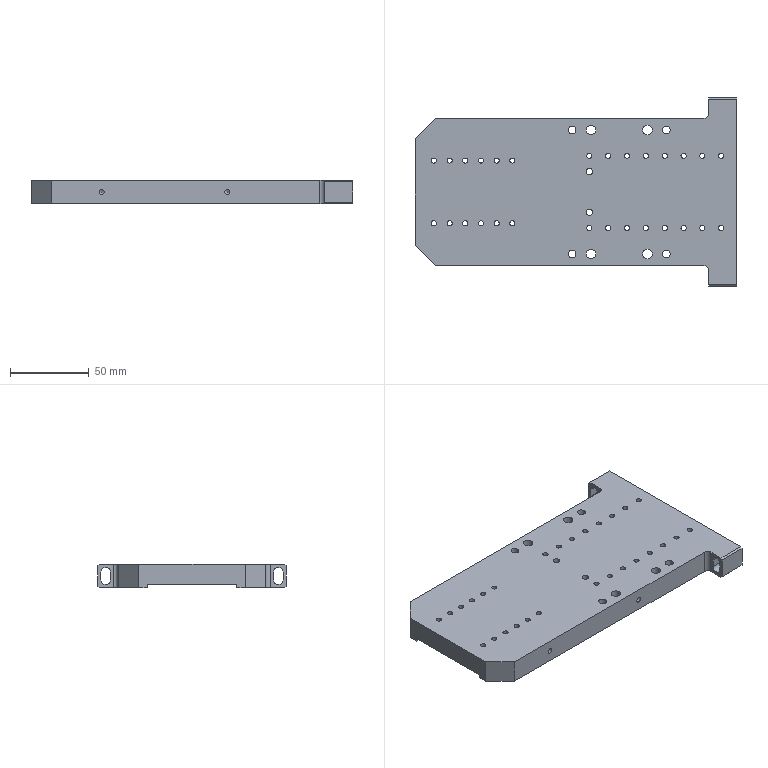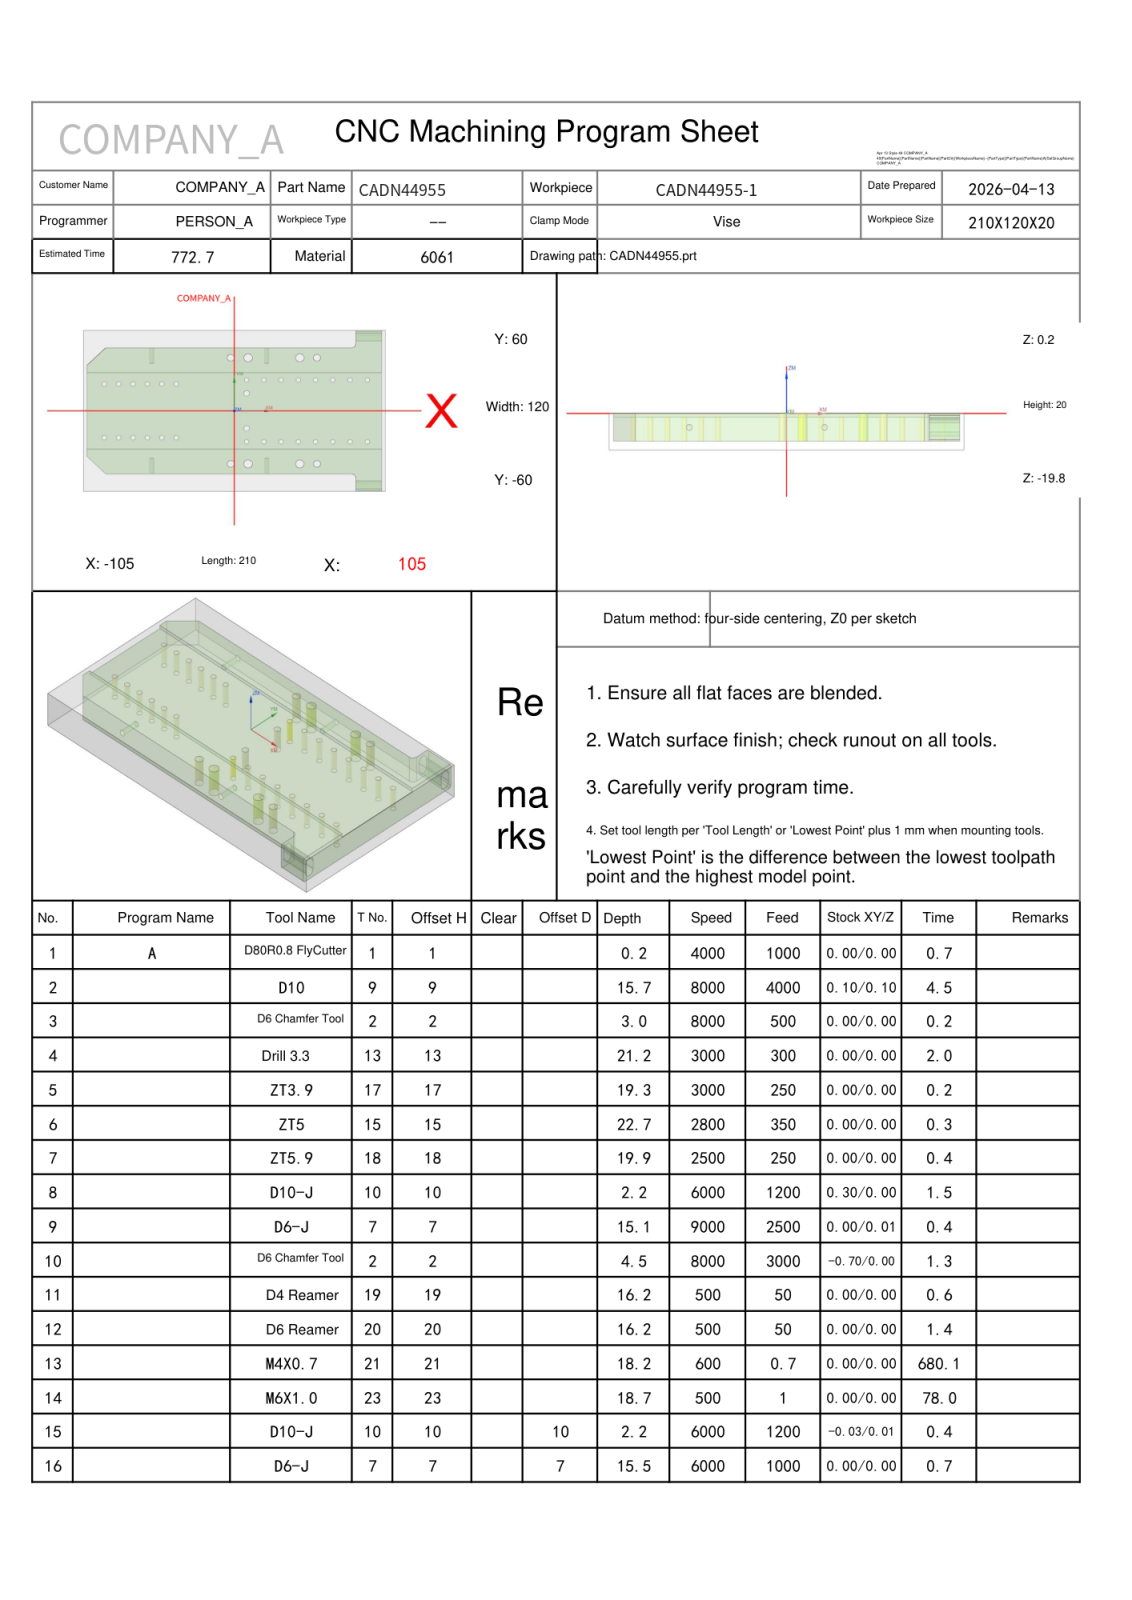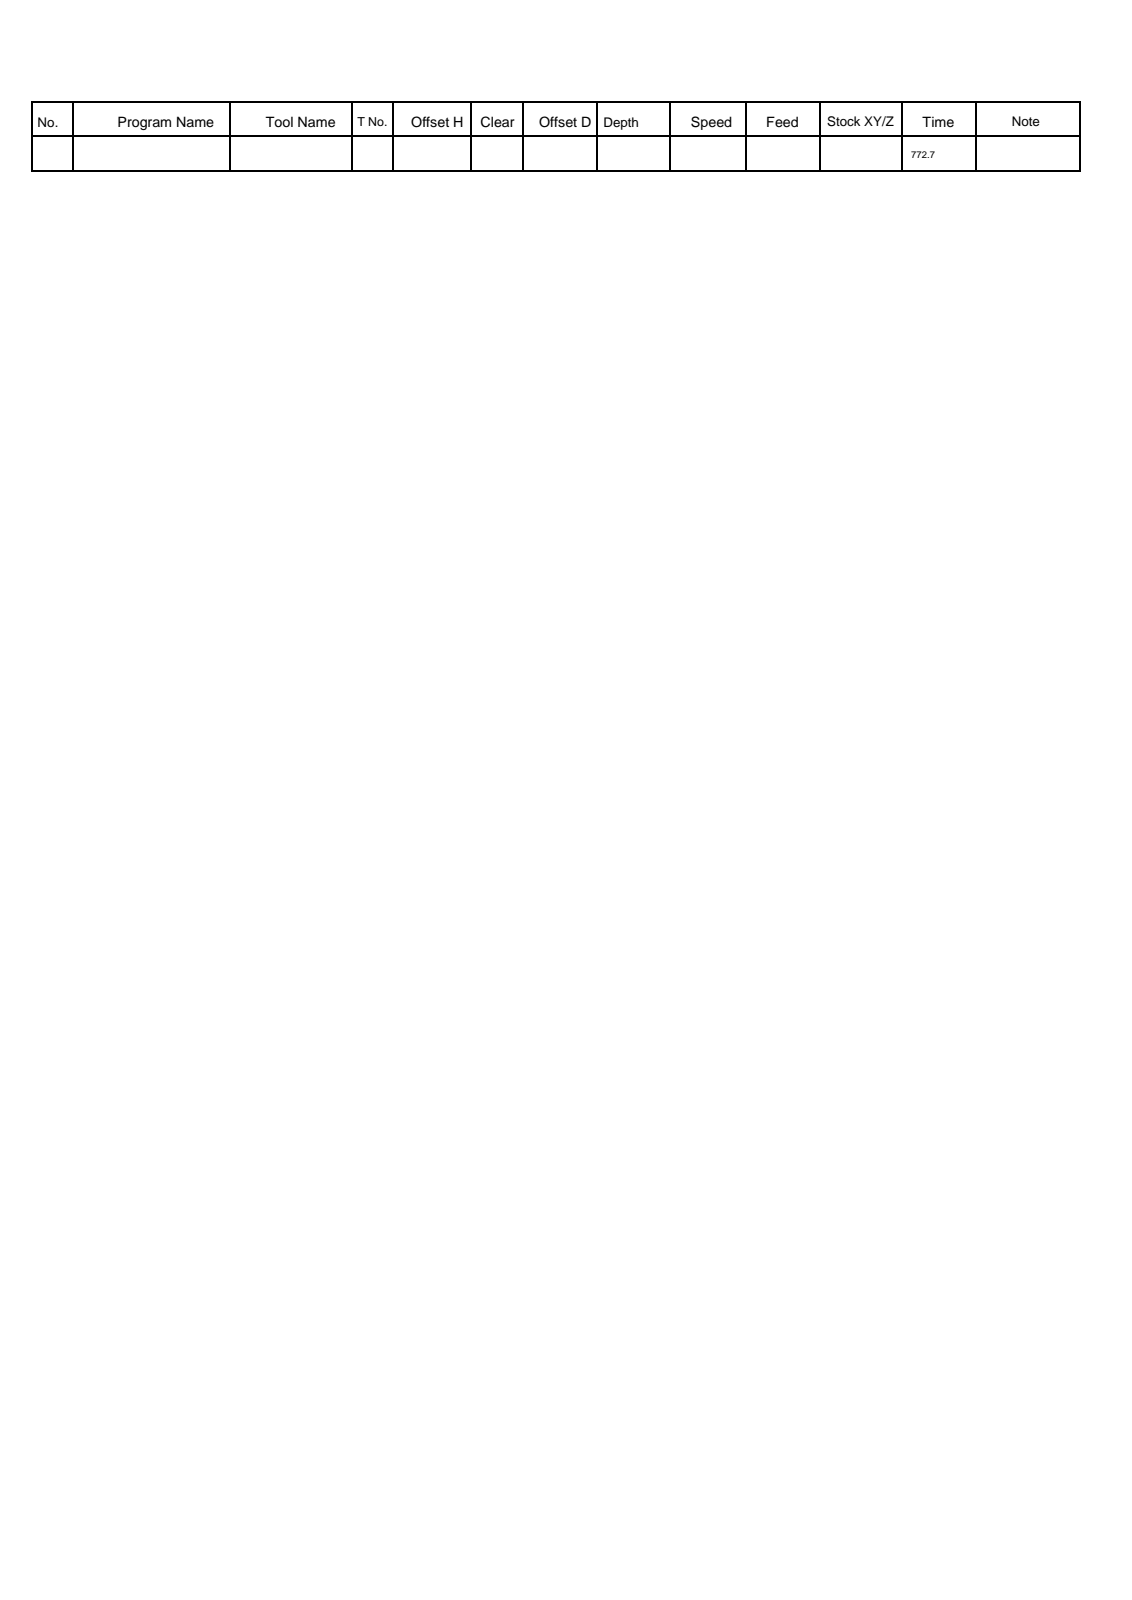NC program | NX | posted by the shop | part box 205 x 120 x 15 mm
Lines 1 to 1265 of 4760:
%
O0001
(Machine time: 1489.33 MIN)
(===Total Tool:13===)
(T1=D80R0.8 FlyCutter D=80.  R=0.8  D-  H01 Z=-0.   )
(T9=D10     D=10.  R=0.   D-  H09 Z=-15.5 )
(T2=D6 ChamferTool   D=6.   R=0.   D-  H02 Z=-4.3  )
(T13=Drill 3.3  D=3.3  DR_a=118 D-  H13 Z=-20.99)
(T17=ZT3.9  D=3.9  DR_a=120 D-  H17 Z=-19.13)
(T15=ZT5    D=5.   DR_a=118 D-  H15 Z=-22.5 )
(T18=ZT5.9  D=5.9  DR_a=120 D-  H18 Z=-19.7 )
(T10=D10-J  D=10.  R=0.   D-  H10 Z=-2.   )
(T7=D6-J    D=6.   R=0.   D-  H07 Z=-15.3 )
(T19=D4 Reamer   D=4.   DR_a=180 D-  H19 Z=-16.  )
(T20=D6 Reamer   D=6.   DR_a=180 D-  H20 Z=-16.  )
(T21=M4X0.7 D=3.3  DR_a=180 D-  H21 Z=-18.  )
(T23=M6X1.0 D=5.   DR_a=180 D-  H23 Z=-18.5 )
G80 G90 G17 G49 G40
G91 G28 Z0
M01
N1 T01 M06
(D80R0.8 FlyCutter  D=80. R=0.8 H=01 ce=0.00 di=0.00)
(MAX_Z=20. MIN_Z=-0. Time=0.66M)
G00 G90 G54 X147.5 Y-33.333 M03 S4000
G43 H01 Z20.
M08
Z2.
G01 Z0.0 F1000.
X142.5
X-142.5
Y33.333
X142.5
X147.5
Z2.
G00 Z20.
G91 G28 Z0.0
M05
M09
G91 G28 Z0.0
M01
N2 T09 M06
(D10  D=10. R=0. H=09 ce=0.12 di=0.10)
(MAX_Z=20. MIN_Z=-15.5 Time=4.44M)
G00 G90 G54 X115.931 Y.933 M03 S8000
G43 H09 Z20.
M08
Z-13.5
G01 X115.832 Y.914 Z-14.125 F4000.
X115.734 Y.895 Z-14.372
X115.636 Y.877 Z-14.554
X115.538 Y.858 Z-14.7
X115.439 Y.839 Z-14.823
X115.341 Y.821 Z-14.928
X115.243 Y.802 Z-15.02
X115.145 Y.783 Z-15.1
X115.046 Y.765 Z-15.17
X114.948 Y.746 Z-15.232
X114.85 Y.727 Z-15.286
X114.752 Y.709 Z-15.333
X114.653 Y.69 Z-15.374
X114.555 Y.671 Z-15.408
X114.457 Y.653 Z-15.436
X114.359 Y.634 Z-15.46
X114.261 Y.615 Z-15.477
X114.162 Y.597 Z-15.49
X114.064 Y.578 Z-15.497
X113.966 Y.559 Z-15.5
X111.852 Y.158
G03 X111.5 Y-.101 I.101 J-.505
X110.862 Y-3.914 I12.263 J-4.012
X110.681 Y-14.084 I285.594 J-10.169
X110.7 Y-17.408 I285.775 J0.0
G01 X110.683 Y-58.128
G02 X106.817 Y-64.032 I-6.644 J.133
X101.024 Y-65.449 I-6.598 J14.422
X91.905 Y-65.715 I-9.119 J156.488
X89.509 Y-65.696 I0.0 J156.754
G01 X-103.13 Y-65.682
G02 X-109.102 Y-61.67 I.144 J6.665
X-110.476 Y-55.702 I15.279 J6.659
X-110.719 Y-46.222 I184.586 J9.48
X-110.699 Y-43.467 I184.829 J0.0
G01 X-110.68 Y58.17
G02 X-106.87 Y63.995 I6.601 J-.16
X-101.239 Y65.427 I6.537 J-13.917
X-92.501 Y65.714 I8.738 J-132.999
X-90.366 Y65.697 I0.0 J-133.286
G01 X103.25 Y65.676
G02 X108.958 Y61.949 I-.203 J-6.546
X110.434 Y56.172 I-13.856 J-6.618
X110.713 Y47.477 I-135.526 J-8.695
X110.697 Y45.378 I-135.804 J0.0
G01 X110.683 Y2.679
G03 X110.095 Y-4.195 I455.395 J-42.432
X109.895 Y-14.598 I270.442 J-10.404
X109.9 Y-16.368 I270.642 J0.0
G01 X109.884 Y-56.108
G02 X107.365 Y-61.553 I-7.562 J.194
G01 X106.934 Y-62.56
X106.12 Y-63.62
X105.06 Y-64.434
X103.825 Y-64.946
X102.498 Y-65.12
X84.221 Y-65.098
G03 X75.842 Y-64.892 I-8.378 J-170.229
X73.989 Y-64.902 I0.0 J-170.435
G01 X-101.208 Y-64.879
G02 X-107.674 Y-60.783 I.383 J7.756
X-109.531 Y-54.375 I14.417 J7.651
X-109.905 Y-45.467 I105.986 J8.909
X-109.892 Y-43.826 I106.359 J0.0
G01 X-109.877 Y56.247
G02 X-105.805 Y62.659 I7.751 J-.424
X-99.391 Y64.529 I7.66 J-14.337
X-90.425 Y64.906 I8.966 J-106.458
X-88.762 Y64.893 I0.0 J-106.835
G01 X83.043 Y64.908
X84.502 Y65.12
X102.502
X103.825 Y64.946
X105.06 Y64.434
G02 X107.707 Y61.406 I-4.202 J-6.345
X109.559 Y54.573 I-16.215 J-8.062
X109.899 Y45.806 I-112.829 J-8.767
X109.892 Y44.502 I-113.169 J0.0
G01 X109.873 Y4.122
G02 X109.322 Y-4.177 I-786.201 J48.07
G03 X109.086 Y-17.016 I349.156 J-12.839
X109.101 Y-20.208 I349.392 J0.0
G01 X109.079 Y-54.268
G02 X107.67 Y-59.053 I-11.286 J.725
G03 X107.603 Y-59.683 I2.925 J-.63
X107.62 Y-60.002 I2.992 J0.0
G01 X107.446 Y-61.325
X107.323 Y-61.621
X107.446 Y-61.325
G03 X107.649 Y-58.872 I-17.171 J2.657
X108.438 Y-50.971 I-39.167 J7.902
X108.432 Y-50.313 I-39.956 J0.0
G01 X108.492 Y-11.541
G02 X109.141 Y2.682 I232.868 J-3.495
G03 X109.263 Y11.371 I-309.22 J8.689
X109.258 Y13.081 I-309.342 J0.0
G01 X109.227 Y47.141
G03 X109.231 Y47.792 I-56.575 J.652
X108.633 Y55.991 I-56.578 J0.0
X107.62 Y59.573 I-19.448 J-3.568
X107.446 Y61.325 I-10.322 J-.143
G01 X106.934 Y62.56
X106.12 Y63.62
X106.934 Y62.56
X107.446 Y61.325
G02 X107.641 Y58.913 I-14.765 J-2.412
X107.638 Y58.591 I-14.961 J0.0
X108.451 Y44.13 I-128.221 J-14.461
X108.445 Y42.88 I-129.034 J0.0
G01 X108.436 Y7.38
G02 X107.915 Y-4.166 I-251.422 J5.565
G03 X107.639 Y-20.142 I462.713 J-15.975
X107.661 Y-24.609 I462.988 J0.0
G01 X107.63 Y-49.609
X107.62 Y-59.205
X107.635 Y1.039
G03 X107.83 Y15.095 I-507.419 J14.056
X107.818 Y18.54 I-507.613 J0.0
G01 X107.782 Y45.08
G03 X107.62 Y50.886 I-539.839 J-12.143
G01 Y58.966
Y.326
G03 X107.795 Y-.055 I.513 J.006
G01 X108.582 Y-.726
X110.082 Y-2.005 Z-15.4
X110.581 Y-2.431
X110.642 Y-2.493
X110.691 Y-2.564
X110.727 Y-2.642
X110.749 Y-2.725
X110.757 Y-2.811
Y-63.265
X110.75 Y-63.442
X110.727 Y-63.618
X110.691 Y-63.792
X110.64 Y-63.962
X110.575 Y-64.127
X110.497 Y-64.286
X110.406 Y-64.438
X110.302 Y-64.582
X110.187 Y-64.717
X110.061 Y-64.842
X109.926 Y-64.957
X109.781 Y-65.059
X104.919 Y-68.204
X104.685 Y-68.348
X104.444 Y-68.48
X104.197 Y-68.6
X103.944 Y-68.707
X103.687 Y-68.803
X103.425 Y-68.885
X103.159 Y-68.955
X102.89 Y-69.012
X102.619 Y-69.056
X102.346 Y-69.086
X102.072 Y-69.103
X101.797 Y-69.106
X101.522 Y-69.096
X87.635 Y-68.257
X87.558 Y-68.246
X87.483 Y-68.223
X87.412 Y-68.189
X87.348 Y-68.144
X87.291 Y-68.089
X86.857 Y-67.598
X85.549 Y-66.122 Z-15.5
X84.756 Y-65.234
X84.498 Y-65.12
G02 X82.23 Y-64.654 I.712 J9.228
G03 X76.11 Y-64.146 I-6.12 J-36.62
X75.677 Y-64.149 I0.0 J-37.127
G01 X65.192 Y-64.1
X-99.188 Y-64.083
G02 X-106.881 Y-59.122 I.265 J8.856
X-108.708 Y-52.442 I16.621 J8.136
X-109.102 Y-43.026 I112.211 J9.416
X-109.091 Y-41.414 I112.606 J0.0
G01 X-109.075 Y54.326
G02 X-104.209 Y61.832 I8.829 J-.393
X-97.624 Y63.687 I8.117 J-16.205
X-88.243 Y64.102 I9.381 J-105.829
X-86.677 Y64.09 I0.0 J-106.244
G01 X81.386 Y64.121
G03 X81.94 Y64.434 I-.337 J1.244
G01 X83.175 Y64.946
X81.94 Y64.434
G02 X80.371 Y63.821 I-1.726 J2.105
X74.324 Y63.468 I-6.047 J51.518
X73.378 Y63.476 I0.0 J51.872
G01 X-88.409 Y63.436
G03 X-89.329 Y63.442 I-.92 J-71.028
X-98.066 Y62.902 I0.0 J-71.034
X-104.129 Y60.744 I1.689 J-14.335
X-107.836 Y54.861 I5.345 J-7.477
X-108.422 Y48.3 I36.385 J-6.561
X-108.42 Y47.857 I36.972 J0.0
G01 X-108.458 Y38.897
X-108.436 Y-43.403
G03 X-108.441 Y-44.251 I73.299 J-.847
X-107.928 Y-52.903 I73.304 J0.0
X-105.841 Y-58.989 I14.732 J1.652
X-99.95 Y-62.817 I7.539 J5.154
X-93.426 Y-63.42 I6.525 J35.016
X-93.028 Y-63.418 I0.0 J35.619
G01 X-83.748 Y-63.46
X73.461 Y-63.485
G02 X74.264 Y-63.479 I.802 J-53.491
X81.184 Y-63.928 I0.0 J-53.497
X81.94 Y-64.434 I-.918 J-2.189
G01 X82.975 Y-64.863
G02 X81.258 Y-63.911 I1.318 J4.401
G03 X77.863 Y-63.021 I-3.975 J-8.239
X69.772 Y-62.664 I-8.091 J-91.655
X68.614 Y-62.671 I0.0 J-92.011
G01 X-91.088 Y-62.636
G02 X-91.803 Y-62.641 I-.714 J43.495
X-98.343 Y-62.147 I0.0 J43.501
X-105.786 Y-56.085 I1.709 J9.7
X-107.353 Y-49.008 I20.895 J8.338
X-107.668 Y-38.964 I159.95 J10.045
X-107.656 Y-37.015 I160.265 J0.0
G01 X-107.638 Y45.765
G02 X-107.645 Y46.57 I46.82 J.805
X-107.176 Y53.182 I46.827 J0.0
X-101.086 Y60.785 I9.739 J-1.56
X-93.848 Y62.367 I8.413 J-21.155
X-84.311 Y62.661 I9.537 J-154.26
X-82.735 Y62.653 I0.0 J-154.555
G01 X72.964 Y62.678
G03 X73.79 Y62.671 I.826 J46.532
X79.707 Y63.049 I0.0 J46.539
X80.696 Y63.381 I-.094 J1.915
G02 X81.641 Y64.205 I2.918 J-2.395
G03 X80.591 Y63.261 I2.125 J-3.419
G02 X77.79 Y62.406 I-3.372 J6.036
X70.488 Y62.026 I-7.302 J69.897
X69.462 Y62.034 I0.0 J70.277
G01 X-85.851 Y61.993
G03 X-86.725 Y61.999 I-.874 J-72.788
X-95.748 Y61.437 I0.0 J-72.794
X-102.039 Y59.205 I1.794 J-15.039
X-106.145 Y52.99 I6.079 J-8.481
X-106.945 Y45.779 I32.106 J-7.211
G01 Y45.77
X-107.045 Y36.293
X-107.446 Y35.325
X-107.62 Y34.002
Y-33.998
G02 X-107.029 Y-40.904 I-44.933 J-7.321
G03 X-106.524 Y-50.157 I89.085 J.226
X-104.493 Y-56.595 I16.391 J1.631
X-98.128 Y-61.11 I8.685 J5.501
X-90.912 Y-61.942 I7.223 J30.952
X-80.866 Y-62.02 I10.047 J639.268
G01 X-79.793
X69.783 Y-62.044
G02 X70.539 Y-62.04 I.757 J-63.139
X78.167 Y-62.502 I0.0 J-63.144
X80.502 Y-63.15 I-.711 J-7.098
G03 X81.26 Y-63.913 I2.302 J1.53
G02 X80.463 Y-63.083 I1.523 J2.262
G03 X77.789 Y-61.951 I-3.637 J-4.869
X70.388 Y-61.289 I-7.401 J-41.012
G01 X70.217
G03 X60.937 Y-61.22 I-9.28 J-617.94
G01 X60.552
X-87.328 Y-61.196
G02 X-88.122 Y-61.202 I-.794 J53.223
X-95.623 Y-60.671 I0.0 J53.229
X-101.926 Y-57.614 I1.526 J11.173
X-105.205 Y-51.275 I9.771 J9.073
X-106.133 Y-43.021 I42.253 J8.927
G03 X-106.48 Y-37.201 I-73.412 J-1.458
G01 X-106.934 Y-36.56
X-107.446 Y-35.325
X-106.934 Y-36.56
G02 X-105.995 Y-38.724 I-2.915 J-2.551
X-105.35 Y-45.495 I-77.079 J-10.758
G03 X-103.956 Y-52.615 I26.177 J1.428
X-96.347 Y-59.496 I10.361 J3.811
X-88.989 Y-60.469 I7.684 J29.797
X-78.716 Y-60.585 I10.273 J454.097
X-76.431 Y-60.579 I0.0 J454.213
G01 X66.43 Y-60.6
G02 X67.397 Y-60.594 I.967 J-76.824
X75.974 Y-61.074 I0.0 J-76.83
X79.855 Y-62.245 I-.984 J-10.28
G01 X80.553 Y-63.195
G02 X79.832 Y-62.15 I8.631 J6.729
G03 X77.024 Y-60.752 I-4.045 J-4.602
X69.831 Y-59.909 I-7.544 J-33.273
X59.103 Y-59.776 I-10.728 J-434.186
X57.351 Y-59.78 I0.0 J-434.319
G01 X-84.049 Y-59.759
G02 X-84.922 Y-59.765 I-.873 J64.215
X-92.987 Y-59.256 I0.0 J64.221
X-99.319 Y-56.758 I1.607 J13.346
X-103.433 Y-50.406 I7.991 J9.685
X-104.605 Y-43.8 I33.341 J9.323
G03 X-105.397 Y-38.476 I-32.057 J-2.043
X-106.121 Y-37.619 I-2.248 J-1.166
G01 X-106.511 Y-37.111
G03 X-105.414 Y-38.335 I7.177 J5.329
G02 X-104.39 Y-41.465 I-7.503 J-4.186
G03 X-103.297 Y-48.009 I134.733 J19.145
X-100.295 Y-54.407 I14.097 J2.712
X-93.545 Y-58.221 I9.312 J8.598
X-85.272 Y-59.068 I8.273 J39.974
G01 X-85.204
G03 X-75.472 Y-59.141 I9.731 J648.808
X-74.004 Y-59.139 I0.0 J648.881
G01 X64.188 Y-59.162
G02 X65.076 Y-59.157 I.888 J-84.294
X74.238 Y-59.656 I0.0 J-84.299
X78.918 Y-61.022 I-1.231 J-12.917
X79.689 Y-61.649 I-1.321 J-2.41
G01 X79.995 Y-62.388
G03 X78.045 Y-60.197 I-3.218 J-.9
X72.886 Y-58.837 I-6.567 J-14.445
X63.127 Y-58.355 I-9.759 J-98.719
X62.203 Y-58.36 I0.0 J-99.2
G01 X-81.348 Y-58.319
G02 X-82.226 Y-58.324 I-.878 J71.523
X-90.688 Y-57.822 I0.0 J71.529
X-97.182 Y-55.498 I1.706 J15.001
X-101.815 Y-49.101 I7.481 J10.294
X-103.379 Y-42.519 I43.605 J13.84
G03 X-104.263 Y-39.477 I-11.593 J-1.72
G01 X-105.508 Y-38.233
G02 X-104.02 Y-39.764 I-27.181 J-27.891
X-102.709 Y-43.303 I-10.452 J-5.885
G03 X-100.951 Y-49.188 I38.014 J8.147
X-92.669 Y-56.47 I11.48 J4.707
X-84.685 Y-57.568 I8.46 J31.951
X-74.579 Y-57.703 I10.105 J377.13
X-72.766 Y-57.699 I0.0 J377.265
G01 X61.555 Y-57.718
G02 X62.627 Y-57.712 I1.072 J-98.534
X72.594 Y-58.217 I0.0 J-98.539
X77.918 Y-59.645 I-1.531 J-16.351
X79.466 Y-60.868 I-1.787 J-3.853
G03 X79.677 Y-61.621 I4.085 J.737
G02 X79.484 Y-60.834 I2.179 J.951
G03 X77.693 Y-59.103 I-3.466 J-1.795
X72.109 Y-57.492 I-7.212 J-14.511
X62.097 Y-56.931 I-10.012 J-89.073
X61.549 Y-56.932 I0.0 J-89.634
G01 X51.672 Y-56.9
X-79.488 Y-56.874
G02 X-80.213 Y-56.877 I-.724 J69.823
X-88.905 Y-56.334 I0.0 J69.826
X-95.748 Y-53.8 I1.857 J15.52
X-100.354 Y-47.64 I8.223 J10.952
X-102.234 Y-42.108 I116.888 J42.797
G01 X-102.686 Y-41.055
X-104.157 Y-39.584
G02 X-102.306 Y-41.514 I-13.524 J-14.817
X-100.576 Y-45.336 I-18.938 J-10.877
G03 X-97.309 Y-51.101 I17.464 J6.086
X-89.992 Y-55.241 I10.243 J9.567
X-81.497 Y-56.165 I8.738 J40.839
X-70.601 Y-56.259 I10.896 J631.817
G01 X-70.378
X59.634 Y-56.278
G02 X60.748 Y-56.272 I1.114 J-105.103
X71.395 Y-56.813 I0.0 J-105.109
X77.233 Y-58.359 I-1.771 J-18.482
X79.379 Y-60.131 I-2.012 J-4.624
G01 X79.504 Y-60.939
G03 X78.15 Y-58.49 I-2.945 J-.03
X73.402 Y-56.509 I-6.904 J-9.867
X64.024 Y-55.577 I-9.803 J-50.957
X52.086 Y-55.458 I-11.938 J-599.558
X50.711 Y-55.46 I0.0 J-599.677
G01 X-77.009 Y-55.436
G02 X-77.906 Y-55.441 I-.898 J74.391
X-87.065 Y-54.875 I0.0 J74.396
X-94.21 Y-52.256 I1.975 J16.443
X-98.948 Y-46.483 I9.134 J12.327
G01 X-100.601 Y-43.14
X-102.58 Y-41.16
G02 X-99.981 Y-43.844 I-24.923 J-26.738
G01 X-97.494 Y-47.666
G03 X-88.243 Y-53.79 I12.311 J8.548
X-79.428 Y-54.725 I9.057 J43.36
X-68.023 Y-54.822 I11.405 J675.763
X-66.228 Y-54.819 I0.0 J675.86
G01 X58.033 Y-54.839
G02 X59.104 Y-54.834 I1.071 J-110.458
X70.279 Y-55.401 I0.0 J-110.463
X76.625 Y-57.05 I-1.995 J-20.712
X79.3 Y-59.262 I-2.353 J-5.57
X79.403 Y-60.036 I-2.851 J-.773
G01 X79.401 Y-60.157
X79.405 Y-59.983
G03 X79.267 Y-58.982 I-3.705 J0.0
X76.855 Y-56.65 I-4.776 J-2.526
X70.751 Y-54.784 I-8.384 J-16.504
X59.806 Y-54.072 I-10.945 J-83.784
G01 X59.61
X49.111 Y-54.02
X-74.789 Y-53.996
G02 X-75.717 Y-54.002 I-.928 J80.218
X-85.166 Y-53.443 I0.0 J80.223
X-90.574 Y-51.979 I2.798 J21.045
X-92.589 Y-51.074 I1.042 J5.018
X-96.547 Y-47.194 I10.791 J14.965
G01 X-100.394 Y-43.347
X-93.122 Y-50.619
X-92.06 Y-51.434
X-90.825 Y-51.946
G03 X-83.736 Y-52.934 I73.517 J501.246
X-72.89 Y-53.375 I10.845 J133.074
X-71.588 Y-53.369 I0.0 J133.515
G01 X56.354 Y-53.399
G02 X57.418 Y-53.394 I1.064 J-119.559
X69.098 Y-53.966 I0.0 J-119.564
X76.095 Y-55.733 I-2.138 J-23.209
X79.219 Y-58.264 I-2.66 J-6.476
G01 X79.38 Y-58.666
Y-59.466
G03 X79.404 Y-59.066 I-3.306 J.4
X79.211 Y-57.948 I-3.33 J0.0
X76.492 Y-55.382 I-5.434 J-3.034
X69.879 Y-53.378 I-9.101 J-18.123
X58.797 Y-52.646 I-11.196 J-85.234
X48.154 Y-52.571 I-10.643 J-753.894
X44.471 Y-52.58 I0.0 J-753.969
G01 X-72.529 Y-52.558
G02 X-73.058 Y-52.559 I-.529 J118.987
X-83.277 Y-52.12 I0.0 J118.988
G01 X-89.502
X62.336 Y-52.145
G02 X72.191 Y-53.257 I-.684 J-50.287
X77.825 Y-55.736 I-2.866 J-14.154
X79.372 Y-57.664 I-2.841 J-3.863
G01 X79.38 Y-58.511
G03 X79.404 Y-58.108 I-3.325 J.402
X79.166 Y-56.868 I-3.35 J0.0
X76.24 Y-54.139 I-5.94 J-3.437
X69.951 Y-52.12 I-9.364 J-18.36
G01 X61.311
X71.451 Y-52.142
G02 X78.297 Y-55.108 I-1.002 J-11.699
X79.38 Y-56.709 I-2.598 J-2.923
G01 Y-57.589
G03 X79.403 Y-57.154 I-4.031 J.435
X79.24 Y-56.013 I-4.055 J0.0
X76.598 Y-53.259 I-5.651 J-2.777
X74.058 Y-52.12 I-6.028 J-10.039
G01 X71.018
G02 X72.359 Y-52.098 I1.34 J-41.191
X74.695 Y-52.164 I0.0 J-41.212
X79.233 Y-55.303 I-1.284 J-6.706
G01 X79.38 Y-55.69
Y-56.57
G03 X79.403 Y-56.135 I-4.042 J.434
X79.236 Y-54.982 I-4.065 J0.0
X76.033 Y-52.12 I-5.032 J-2.409
G01 X74.273
G02 X75.051 Y-52.101 I.778 J-15.782
X76.41 Y-52.159 I0.0 J-15.801
X79.36 Y-54.616 I-1.19 J-4.428
G01 X79.38 Y-55.6
G03 X79.401 Y-55.172 I-4.406 J.428
X79.289 Y-54.183 I-4.427 J0.0
X77.23 Y-52.12 I-3.257 J-1.192
G01 X76.11
G02 X76.596 Y-52.102 I.486 J-6.664
X77.585 Y-52.176 I0.0 J-6.682
X79.38 Y-53.906 I-.835 J-2.662
G01 Y-54.626
G03 X79.403 Y-54.268 I-2.732 J.357
X79.187 Y-53.199 I-2.755 J0.0
X77.977 Y-52.12 I-1.813 J-.815
G01 X77.257
G02 X77.599 Y-52.1 I.341 J-2.851
X78.344 Y-52.198 I0.0 J-2.872
X79.38 Y-53.318 I-.656 J-1.647
G01 Y-53.878
G03 X79.405 Y-53.583 I-1.727 J.295
X78.938 Y-52.393 I-1.752 J0.0
X78.256 Y-52.097 I-.682 J-.64
X78.051 Y-52.12 I0.0 J-.935
G02 X78.288 Y-52.095 I.236 J-1.109
X79.38 Y-52.926 I0.0 J-1.134
G01 Y-53.246
G03 X79.404 Y-53.031 I-.943 J.215
X78.762 Y-52.12 I-.968 J0.0
G01 X78.522
X78.648 Y-52.109
G02 X79.287 Y-52.459 I0.0 J-.759
X79.374 Y-52.752 I-.454 J-.293
X78.833 Y-53.293 I-.541 J0.0
X78.457 Y-53.141 I0.0 J.541
X78.21 Y-52.668 I.33 J.473
X78.311 Y-52.341 I.577 J0.0
X78.745 Y-52.126 I.434 J-.328
G01 X78.85 Y-52.136
G02 X79.393 Y-52.763 I-.091 J-.627
G01 X79.38 Y-52.889
G02 X79.153 Y-53.311 I-.512 J.004
G01 X77.215 Y-54.588
X77.071 Y-54.65
X76.915 Y-54.671
X76.815 Y-54.666 Z-15.497
X76.716 Y-54.662 Z-15.49
X76.616 Y-54.658 Z-15.477
X76.516 Y-54.653 Z-15.46
X76.416 Y-54.649 Z-15.436
X76.316 Y-54.645 Z-15.408
X76.216 Y-54.64 Z-15.374
X76.116 Y-54.636 Z-15.333
X76.016 Y-54.632 Z-15.286
X75.916 Y-54.628 Z-15.232
X75.816 Y-54.623 Z-15.17
X75.716 Y-54.619 Z-15.1
X75.617 Y-54.615 Z-15.02
X75.517 Y-54.61 Z-14.928
X75.417 Y-54.606 Z-14.823
X75.317 Y-54.602 Z-14.7
X75.217 Y-54.598 Z-14.554
X75.117 Y-54.593 Z-14.372
X75.017 Y-54.589 Z-14.125
X74.917 Y-54.585 Z-13.5
G00 Z20.
X-108.859 Y38.353
Z-13.5
G01 X-108.897 Y38.26 Z-14.125
X-108.936 Y38.168 Z-14.372
X-108.974 Y38.076 Z-14.554
X-109.012 Y37.983 Z-14.7
X-109.05 Y37.891 Z-14.823
X-109.089 Y37.799 Z-14.928
X-109.127 Y37.706 Z-15.02
X-109.165 Y37.614 Z-15.1
X-109.204 Y37.521 Z-15.17
X-109.242 Y37.429 Z-15.232
X-109.28 Y37.337 Z-15.286
X-109.318 Y37.244 Z-15.333
X-109.357 Y37.152 Z-15.374
X-109.395 Y37.059 Z-15.408
X-109.433 Y36.967 Z-15.436
X-109.471 Y36.875 Z-15.46
X-109.51 Y36.782 Z-15.477
X-109.548 Y36.69 Z-15.49
X-109.586 Y36.598 Z-15.497
X-109.624 Y36.505 Z-15.5
X-109.663 Y36.312
G03 X-109.158 Y35.807 I.505 J0.0
G01 X-109.105 Y35.81
X-107.458 Y35.984
G03 X-107.045 Y36.293 I-.056 J.506
X-106.394 Y39.849 I-10.75 J3.805
G02 X-105.997 Y48.063 I768.757 J-33.005
X-104.608 Y54.112 I17.525 J-.839
X-98.413 Y59.546 I9.736 J-4.851
X-90.974 Y60.962 I8.583 J-24.828
X-80.172 Y61.232 I10.802 J-215.923
X-77.539 Y61.216 I0.0 J-216.193
G01 X69.524 Y61.239
G03 X70.368 Y61.232 I.844 J58.293
X77.514 Y61.672 I0.0 J58.299
X79.934 Y62.398 I-.878 J7.325
G01 X80.65 Y63.322
G02 X79.827 Y62.264 I-8.197 J5.529
X76.739 Y61.133 I-3.955 J6.019
X69.431 Y60.617 I-7.308 J51.415
X69.025 Y60.618 I0.0 J51.931
G01 X60.769 Y60.578
X-82.951 Y60.556
G03 X-83.951 Y60.562 I-.999 J-80.413
X-93.33 Y60.013 I0.0 J-80.419
X-99.88 Y57.82 I1.84 J-16.376
X-104.534 Y51.224 I6.193 J-9.31
X-105.501 Y44.265 I31.378 J-7.907
G02 X-106.035 Y38.132 I-50.522 J1.305
X-106.217 Y37.494 I-10.13 J2.552
G01 X-106.934 Y36.56
G03 X-105.71 Y38.436 I-5.228 J4.747
X-104.846 Y43.309 I-20.078 J6.075
G02 X-103.895 Y49.864 I41.493 J-2.671
X-96.457 Y58.065 I11.168 J-2.655
X-88.779 Y59.516 I8.857 J-25.828
X-77.719 Y59.792 I11.06 J-221.44
X-75.024 Y59.776 I0.0 J-221.716
G01 X67.2 Y59.802
G03 X67.946 Y59.798 I.746 J64.012
X75.842 Y60.287 I0.0 J64.016
X79.445 Y61.473 I-1.022 J9.171
G01 X79.736 Y61.764
X80.066 Y62.56
G02 X79.532 Y61.452 I-3.753 J1.126
X76.69 Y60.039 I-4.069 J4.619
X70.036 Y59.262 I-7.081 J31.763
X59.927 Y59.136 I-10.109 J403.923
X58.77 Y59.137 I0.0 J404.05
G01 X-81.05 Y59.111
G03 X-81.842 Y59.114 I-.792 J-79.936
X-91.268 Y58.557 I0.0 J-79.94
X-97.981 Y56.342 I1.956 J-17.215
X-102.978 Y49.562 I6.422 J-9.964
X-104.199 Y43.044 I37.524 J-10.399
G02 X-105.182 Y38.595 I-18.089 J1.667
G01 X-106.119 Y37.622
G03 X-104.767 Y39.114 I-5.29 J6.148
X-103.551 Y43.037 I-12.276 J5.959
G02 X-102.179 Y48.926 I42.006 J-6.676
X-94.352 Y56.682 I11.577 J-3.856
X-86.499 Y58.085 I9.05 J-27.956
X-75.353 Y58.35 I11.147 J-234.866
X-72.744 Y58.335 I0.0 J-235.131
G01 X64.408 Y58.357
G03 X65.259 Y58.352 I.851 J80.669
X74.016 Y58.829 I0.0 J80.674
X78.593 Y60.178 I-1.226 J12.601
X79.483 Y60.938 I-1.04 J2.117
G02 X79.708 Y61.695 I3.165 J-.528
G03 X79.487 Y60.883 I2.237 J-1.045
G02 X77.604 Y59.36 I-3.317 J2.175
X72.069 Y58.077 I-6.686 J16.271
X62.16 Y57.694 I-9.909 J127.977
X60.597 Y57.704 I0.0 J128.36
G01 X-78.152 Y57.676
G03 X-79.173 Y57.681 I-1.021 J-90.433
X-89.012 Y57.145 I0.0 J-90.438
X-96.154 Y54.887 I1.923 J-18.51
X-101.482 Y48.079 I6.69 J-10.725
X-103.094 Y42.157 I64.267 J-20.676
G02 X-103.952 Y39.789 I-11.697 J2.898
G01 X-105.083 Y38.657
G03 X-103.38 Y40.487 I-8.451 J9.576
X-101.996 Y43.879 I-13.92 J7.656
G02 X-99.783 Y49.459 I26.203 J-7.165
X-92.085 Y55.38 I11.353 J-6.795
X-83.81 Y56.685 I9.322 J-32.236
X-72.512 Y56.907 I11.298 J-287.208
X-69.973 Y56.896 I0.0 J-287.43
G01 X62.725 Y56.92
G03 X63.554 Y56.916 I.829 J82.616
X72.963 Y57.454 I0.0 J82.62
X78.039 Y58.973 I-1.486 J14.206
X79.38 Y60.145 I-1.78 J3.388
G01 X79.516 Y61.035
G02 X79.287 Y59.887 I-3.258 J.053
X76.804 Y57.994 I-4.275 J3.031
X70.579 Y56.637 I-7.535 J19.615
X60.479 Y56.26 I-10.099 J135.124
X59.234 Y56.266 I0.0 J135.501
G01 X-76.491 Y56.231
G03 X-77.371 Y56.235 I-.879 J-87.397
X-87.349 Y55.664 I0.0 J-87.401
X-94.678 Y53.285 I2.081 J-18.892
X-100.023 Y46.916 I7.442 J-11.673
G01 X-102.065 Y41.9
X-102.319 Y41.422
X-103.733 Y40.008
G03 X-101.648 Y42.18 I-16. J17.44
X-99.559 Y46.066 I-32.143 J19.784
G02 X-93.913 Y52.369 I13.493 J-6.407
X-86.421 Y54.807 I9.915 J-17.739
X-76.179 Y55.428 I10.242 J-84.09
X-75.407 Y55.425 I0.0 J-84.711
G01 X-64.447 Y55.457
X60.569 Y55.477
G03 X61.509 Y55.473 I.94 J94.593
X71.612 Y56.014 I0.0 J94.598
X77.326 Y57.604 I-1.705 J17.188
X79.353 Y59.378 I-1.893 J4.209
G01 X79.412 Y60.24
X79.37 Y59.343
G02 X77.656 Y57.427 I-3.601 J1.496
X72.163 Y55.568 I-7.399 J12.819
X62.218 Y54.87 I-9.945 J70.509
G01 X62.058
X52.929 Y54.817
X-74.331 Y54.791
G03 X-75.201 Y54.795 I-.87 J-93.644
X-85.35 Y54.243 I0.0 J-93.648
X-93.021 Y51.873 I2.12 J-20.453
X-98.588 Y46.112 I8.235 J-13.529
G01 X-99.96 Y43.78
X-101.997 Y41.744
G03 X-98.515 Y45.304 I-45.035 J47.516
G02 X-94.453 Y49.594 I21.211 J-16.021
G03 X-92.06 Y51.434 I-32.602 J44.866
G02 X-83.097 Y53.582 I11.028 J-26.246
X-72.132 Y54.011 I10.965 J-139.739
X-70.709 Y54.004 I0.0 J-140.169
G01 X58.572 Y54.035
G03 X59.632 Y54.03 I1.06 J105.937
X70.432 Y54.582 I0.0 J105.942
X76.828 Y56.301 I-1.865 J19.698
X79.328 Y58.444 I-2.408 J5.337
X79.401 Y59.092 I-2.834 J.648
X79.38 Y59.438 I-2.907 J0.0
G02 X79.399 Y59.073 I-3.583 J-.365
X79.309 Y58.275 I-3.602 J0.0
X77.031 Y56.002 I-4.554 J2.285
X70.875 Y54.099 I-8.253 J15.796
X60.144 Y53.418 I-10.731 J84.137
G01 X59.753 Y53.419
X50.368 Y53.377
X-72.392 Y53.35
G03 X-73.381 Y53.355 I-.99 J-97.572
X-84.527 Y52.717 I0.0 J-97.577
X-87.636 Y52.12 I11.839 J-70.062
X-88.411 Y52.14 I-.775 J-15.07
X-90.825 Y51.946 I0.0 J-15.09
G02 X-88.411 Y52.14 I2.414 J-14.895
X-87.636 Y52.12 I0.0 J-15.09
G03 X-86.766 Y52.117 I.87 J108.81
X-79.449 Y52.363 I0.0 J108.813
G02 X-63.845 Y52.596 I15.604 J-522.137
X-59.291 Y52.576 I0.0 J-522.37
G01 X57.294 Y52.6
G03 X58.308 Y52.595 I1.015 J108.599
X69.198 Y53.142 I0.0 J108.604
X76.226 Y54.91 I-1.933 J22.539
X79.28 Y57.396 I-2.697 J6.432
G01 X79.38 Y57.678
Y58.638
G02 X79.399 Y58.213 I-4.796 J-.425
X79.316 Y57.324 I-4.815 J0.0
X77.133 Y54.979 I-4.725 J2.21
X70.93 Y52.844 I-8.613 J14.945
X63.548 Y52.12 I-9.487 J58.713
G01 X-84.532
G02 X-85.029 Y52.535 I.001 J.507
G01 X-85.292 Y53.99
X-85.3 Y54.079
G02 X-84.795 Y54.585 I.505 J0.0
G01 X-84.695 Z-15.497
X-84.595 Z-15.49
X-84.495 Z-15.477
X-84.395 Z-15.46
X-84.295 Z-15.436
X-84.195 Z-15.408
X-84.095 Z-15.374
X-83.995 Z-15.333
X-83.895 Z-15.286
X-83.795 Z-15.232
X-83.695 Z-15.17
X-83.595 Z-15.1
X-83.495 Z-15.02
X-83.395 Z-14.928
X-83.295 Z-14.823
X-83.195 Z-14.7
X-83.095 Z-14.554
X-82.995 Z-14.372
X-82.895 Z-14.125
X-82.795 Z-13.5
G00 Z20.
X60.813
Z-13.5
G01 X60.913 Z-14.125
X61.013 Z-14.372
X61.113 Z-14.554
X61.213 Z-14.7
X61.313 Z-14.823
X61.413 Z-14.928
X61.513 Z-15.02
X61.613 Z-15.1
X61.713 Z-15.17
X61.813 Z-15.232
X61.913 Z-15.286
X62.013 Z-15.333
X62.113 Z-15.374
X62.213 Z-15.408
X62.313 Z-15.436
X62.413 Z-15.46
X62.513 Z-15.477
X62.613 Z-15.49
X62.713 Z-15.497
X62.813 Z-15.5
G02 X63.317 Y54.079 I-.001 J-.505
G01 X63.307 Y53.979
X63.053 Y52.725
X63.043 Y52.625
G03 X63.548 Y52.12 I.505 J0.0
X65.997 Y52.096 I2.449 J122.83
X70.197 Y52.167 I0.0 J122.854
X77.472 Y54.535 I-1.051 J15.59
X79.359 Y56.561 I-2.915 J4.607
G01 X79.38 Y57.628
G02 X79.398 Y57.203 I-4.971 J-.425
X79.317 Y56.307 I-4.989 J0.0
X77.045 Y53.825 I-4.944 J2.247
X72.885 Y52.12 I-7.263 J11.79
G01 X69.445
G03 X70.221 Y52.119 I.776 J230.995
X73.977 Y52.149 I0.0 J230.996
X79.127 Y55.104 I-.931 J7.588
X79.38 Y55.644 I-1.538 J1.051
G01 Y56.604
G02 X79.399 Y56.172 I-4.855 J-.432
X79.316 Y55.273 I-4.875 J0.0
X76.838 Y52.713 I-4.796 J2.164
X75.461 Y52.12 I-4.194 J7.84
G01 X73.541
G03 X74.447 Y52.101 I.905 J21.04
X76.135 Y52.168 I0.0 J21.059
X79.351 Y54.542 I-1.024 J4.753
G01 X79.38 Y55.633
G02 X79.401 Y55.199 I-4.49 J-.434
X79.312 Y54.306 I-4.511 J0.0
X76.902 Y52.12 I-3.666 J1.62
G01 X75.702
G03 X76.253 Y52.101 I.552 J8.186
X77.431 Y52.186 I0.0 J8.204
X79.368 Y53.805 I-.768 J2.889
G01 X79.38 Y54.669
G02 X79.399 Y54.305 I-3.467 J-.364
X79.31 Y53.521 I-3.486 J0.0
X77.793 Y52.12 I-2.306 J.976
G01 X76.993
G03 X77.383 Y52.099 I.39 J3.572
X78.309 Y52.22 I0.0 J3.594
X79.38 Y53.291 I-.521 J1.592
G01 Y53.851
G02 X79.405 Y53.568 I-1.591 J-.283
X79.179 Y52.744 I-1.615 J0.0
X78.077 Y52.101 I-1.102 J.624
X77.861 Y52.12 I0.0 J1.266
G03 X78.125 Y52.096 I.263 J1.429
X79.337 Y52.748 I0.0 J1.453
X79.38 Y53.223 I-3.338 J.543
G01 X79.402 Y53.025
G02 X78.487 Y52.11 I-.915 J0.0
G01 X78.354 Y52.12
G03 X78.564 Y52.095 I.209 J.867
X79.299 Y52.483 I0.0 J.892
X79.367 Y52.748 I-.482 J.265
X78.817 Y53.298 I-.55 J0.0
X78.435 Y53.143 I0.0 J-.55
X78.196 Y52.685 I.321 J-.458
X78.756 Y52.125 I.559 J0.0
G01 X78.762
G03 X79.402 Y52.799 I-.035 J.674
G01 X79.38 Y52.969
G03 X79.145 Y53.396 I-.511 J-.003
G01 X77.209 Y54.619
X77.067 Y54.678
X76.915 Y54.697
X76.816 Y54.692 Z-15.497
X76.716 Y54.688 Z-15.49
X76.616 Y54.683 Z-15.477
X76.516 Y54.678 Z-15.46
X76.416 Y54.674 Z-15.436
X76.316 Y54.669 Z-15.408
X76.216 Y54.664 Z-15.374
X76.116 Y54.66 Z-15.333
X76.016 Y54.655 Z-15.286
X75.916 Y54.65 Z-15.232
X75.817 Y54.646 Z-15.17
X75.717 Y54.641 Z-15.1
X75.617 Y54.637 Z-15.02
X75.517 Y54.632 Z-14.928
X75.417 Y54.627 Z-14.823
X75.317 Y54.623 Z-14.7
X75.217 Y54.618 Z-14.554
X75.117 Y54.613 Z-14.372
X75.017 Y54.609 Z-14.125
X74.918 Y54.604 Z-13.5
G00 Z20.
X-99.904 Y47.322
Z-13.5
G01 X-99.975 Y47.252 Z-14.125
X-100.045 Y47.181 Z-14.372
X-100.116 Y47.11 Z-14.554
X-100.187 Y47.039 Z-14.7
X-100.257 Y46.969 Z-14.823
X-100.328 Y46.898 Z-14.928
X-100.399 Y46.827 Z-15.02
X-100.47 Y46.757 Z-15.1
X-100.54 Y46.686 Z-15.17
X-100.611 Y46.615 Z-15.232
X-100.682 Y46.544 Z-15.286
X-100.752 Y46.474 Z-15.333
X-100.823 Y46.403 Z-15.374
X-100.894 Y46.332 Z-15.408
X-100.965 Y46.262 Z-15.436
X-101.035 Y46.191 Z-15.46
X-101.106 Y46.12 Z-15.477
X-101.177 Y46.049 Z-15.49
X-101.247 Y45.979 Z-15.497
X-101.318 Y45.908 Z-15.5
G03 X-101.466 Y45.551 I.357 J-.357
X-101.119 Y45.071 I.505 J0.0
G01 X-99.57 Y44.563
X-99.414 Y44.538
G03 X-99.055 Y44.685 I0.0 J.509
G01 X-93.342 Y50.399
G03 X-93.194 Y50.756 I-.359 J.357
X-93.277 Y51.032 I-.507 J0.0
G01 X-94.399 Y52.746
X-94.454 Y52.83 Z-15.497
X-94.509 Y52.913 Z-15.49
X-94.563 Y52.997 Z-15.477
X-94.618 Y53.08 Z-15.46
X-94.673 Y53.164 Z-15.436
X-94.728 Y53.248 Z-15.408
X-94.783 Y53.331 Z-15.374
X-94.837 Y53.415 Z-15.333
X-94.892 Y53.499 Z-15.286
X-94.947 Y53.582 Z-15.232
X-95.002 Y53.666 Z-15.17
X-95.057 Y53.75 Z-15.1
X-95.111 Y53.833 Z-15.02
X-95.166 Y53.917 Z-14.928
X-95.221 Y54.001 Z-14.823
X-95.276 Y54.084 Z-14.7
X-95.331 Y54.168 Z-14.554
X-95.385 Y54.252 Z-14.372
X-95.44 Y54.335 Z-14.125
X-95.495 Y54.419 Z-13.5
G00 Z20.
G00 G90 X110.5 Y0.0 M03 S6000
Z20.
Z.025
G01 Z-.475 F3500.
X103.5
Y-23.4
X-103.5
Y23.4
X103.5
Y0.0
X96.5
Y-16.4
X-96.5
Y16.4
X96.5
Y0.0
X89.5
Y-9.4
X-89.5
Y9.4
X89.5
Y0.0
X82.5
Y-2.4
X-82.5
Y2.4
X82.5
Y0.0
Y-.5
Z.025
G00 Z.5
X110.5 Y0.0
Z-.45
G01 Z-.95
X103.5
Y-23.4
X-103.5
Y23.4
X103.5
Y0.0
X96.5
Y-16.4
X-96.5
Y16.4
X96.5
Y0.0
X89.5
Y-9.4
X-89.5
Y9.4
X89.5
Y0.0
X82.5
Y-2.4
X-82.5
Y2.4
X82.5
Y0.0
Y-.5
Z-.45
G00 Z.025
X110.5 Y0.0
Z-.925
G01 Z-1.425
X103.5
Y-23.4
X-103.5
Y23.4
X103.5
Y0.0
X96.5
Y-16.4
X-96.5
Y16.4
X96.5
Y0.0
X89.5
Y-9.4
X-89.5
Y9.4
X89.5
Y0.0
X82.5
Y-2.4
X-82.5
Y2.4
X82.5
Y0.0
Y-.5
Z-.925
G00 Z-.45
X110.5 Y0.0
Z-1.4
G01 Z-1.9
X103.5
Y-23.4
X-103.5
Y23.4
X103.5
Y0.0
X96.5
Y-16.4
X-96.5
Y16.4
X96.5
Y0.0
X89.5
Y-9.4
X-89.5
Y9.4
X89.5
Y0.0
X82.5
Y-2.4
X-82.5
Y2.4
X82.5
Y0.0
Y-.5
Z-1.4
G00 Z20.
G91 G28 Z0.0
M05
M09
G91 G28 Z0.0
M01
N3 T02 M06
(D6 ChamferTool  D=6. R=0. H=02 ce=0.00 di=0.10)
(MAX_Z=20. MIN_Z=-2.8 Time=0.18M)
G00 G90 G54 X92.5 Y23. M03 S8000
G43 H02 Z20.
M08
G98 G81 X92.5 Y23. Z-2.8 R-1. F500.
X80.5
X68.5
X56.5
X57.5 Y39.5 Z-.8 R1.
X45.5
X44.5 Y23. Z-2.8 R-1.
X32.5
X20.5
X8.5 Y13.
Y23.
X9.5 Y39.5 Z-.8 R1.
X-2.5
X-40.5 Y20. Z-2.8 R-1.
X-50.5
X-60.5
X-70.5
X-80.5
X-90.5
Y-20.
X-80.5
X-70.5
X-60.5
X-50.5
X-40.5
X-2.5 Y-39.5 Z-.8 R1.
X9.5
X8.5 Y-23. Z-2.8 R-1.
Y-13.
X20.5 Y-23.
X32.5
X44.5
X45.5 Y-39.5 Z-.8 R1.
X57.5
X56.5 Y-23. Z-2.8 R-1.
X68.5
X80.5
X92.5
G80
G00 Z20.
G91 G28 Z0.0
M05
M09
G91 G28 Z0.0
M01
N4 T13 M06
(Drill 3.3 D=3.3 DR_a=118 H=13)
(MAX_Z=20. MIN_Z=-20.99 Time=1.91M)
G00 G90 G54 X-40.5 Y20. M03 S3000
G43 H13 Z20.
M08
G98 G83 X-40.5 Y20. Z-20.991 R-1. F300. Q2.
X-50.5
X-60.5
X-70.5
X-80.5
X-90.5
Y-20.
X-80.5
X-70.5
X-60.5
X-50.5
X-40.5
X8.5 Y-23.
X20.5
X32.5
X44.5
X56.5
X68.5
X80.5
X92.5
Y23.
X80.5
X68.5
X56.5
X44.5
X32.5
X20.5
X8.5
G80
G00 Z20.
G91 G28 Z0.0
M05
M09
G91 G28 Z0.0
M01
N5 T17 M06
(ZT3.9 D=3.9 DR_a=120 H=17)
(MAX_Z=20. MIN_Z=-19.13 Time=0.15M)
G00 G90 G54 X8.5 Y-13. M03 S3000
G43 H17 Z20.
M08
G98 G83 X8.5 Y-13. Z-19.126 R-1. F250. Q2.
Y13.
G80
G00 Z20.
G91 G28 Z0.0
M05
M09
G91 G28 Z0.0
M01
N6 T15 M06
(ZT5 D=5. DR_a=118 H=15)
(MAX_Z=20. MIN_Z=-22.5 Time=0.29M)
G00 G90 G54 X57.5 Y-39.5 M03 S2800
G43 H15 Z20.
M08
G98 G83 X57.5 Y-39.5 Z-22.502 R1. F350. Q3.
X-2.5
Y39.5
X57.5
G80
G00 Z20.
G91 G28 Z0.0
M05
M09
G91 G28 Z0.0
M01
N7 T18 M06
(ZT5.9 D=5.9 DR_a=120 H=18)
(MAX_Z=20. MIN_Z=-19.7 Time=0.35M)
G00 G90 G54 X45.5 Y-39.5 M03 S2500
G43 H18 Z20.
M08
G98 G83 X45.5 Y-39.5 Z-19.703 R1. F250. Q2.
X9.5
Y39.5
X45.5
G80
G00 Z20.
G91 G28 Z0.0
M05
M09
G91 G28 Z0.0
M01
N8 T10 M06
(D10-J  D=10. R=0. H=10 ce=0.30 di=0.00)
(MAX_Z=20. MIN_Z=-2. Time=1.49M)
G00 G90 G54 X110.8 Y-23.199 M03 S6000
G43 H10 Z20.
M08
Z-1.5
G01 Z-2. F1200.
X107.5
X-107.5
Y-16.571
X107.5
Y-9.942
X-107.5
Y-3.314
X107.5
Y3.315
X-107.5
Y9.943
X107.5
Y16.572
X-107.5
Y23.2
X107.5
X110.8
Z-1.5
G00 Z20.
G91 G28 Z0.0
M05
M09
G91 G28 Z0.0
M01